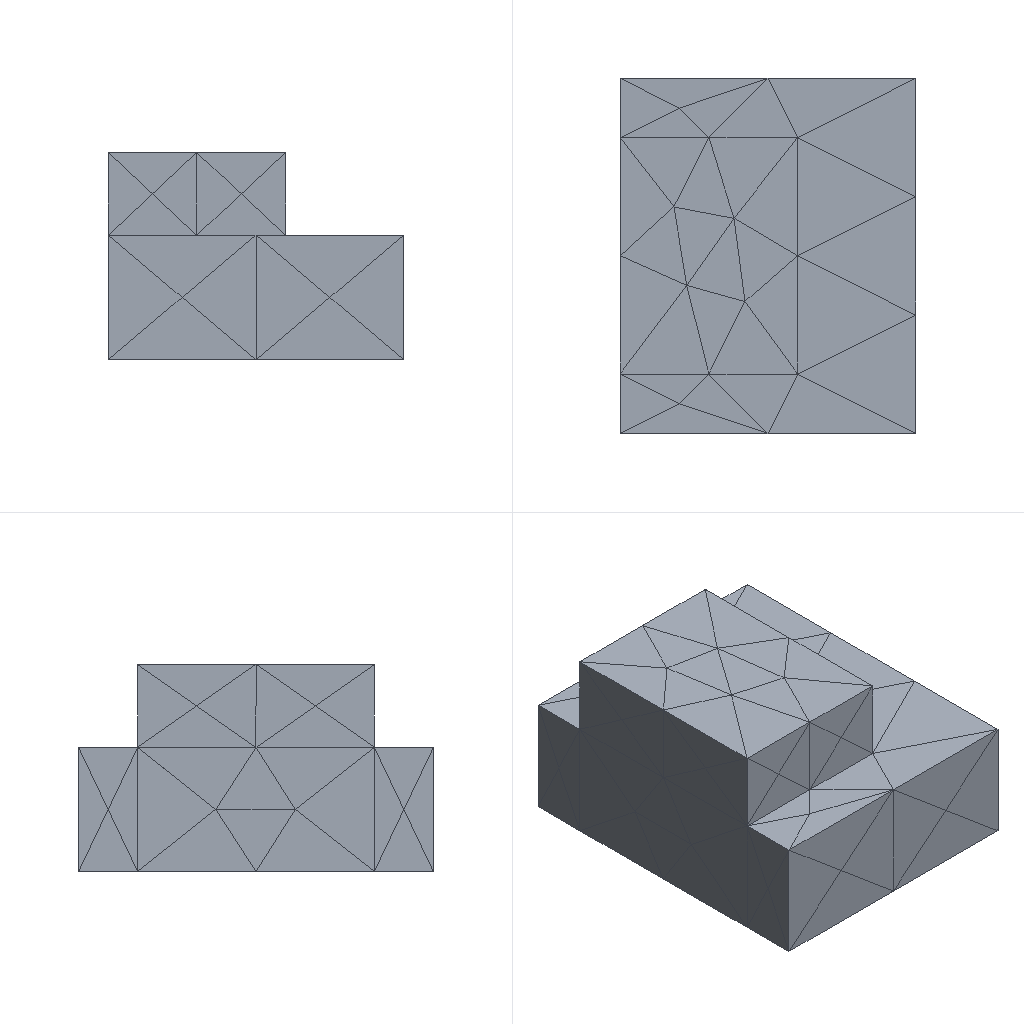Simulation study | ansys mapdl
Set-up summary:
category,name,step,type,value,unit,region
solver,ansys_mapdl
units,mm-N-s-tonne (MPa),,inferred,E=210000 density=
analysis,model,,static
mesh,nodes,,,421
mesh,elements,,,202
element_type,SOLID187,,,202
material,mat 1,,E,210000
material,mat 1,,nu,0.3
load,,model,body load temp,,,all
load,,model,force,"1000 [dir=(0, 0, -1) n=96]",,node list
bc,,model,fixed,"[dofs=UX,UY,UZ n=566]",,node list
Ansys APDL input file, long lists of numbers shortened:
/COM,ANSYS RELEASE 2026 R1           BUILD 26.1      UP20260202       09:11:41
/PREP7
/NOPR
/TITLE,2
ANTYPE, 0
*IF,_CDRDOFF,EQ,1,THEN     !if solid model was read in
_CDRDOFF=             !reset flag, numoffs already performed
*ELSE              !offset database for the following FE model
NUMOFF,NODE,      421
NUMOFF,ELEM,      202
NUMOFF,MAT ,        1
NUMOFF,TYPE,        1
*ENDIF
*SET,_RETURN ,  0.
*SET,_STATUS ,  0.
*SET,_UIQR   ,  96.
*SET,__FLOATPARAMETER__,  421.
DOF,DELETE
ETBLOCK,        1,        1
(2i9,19a9)
        1      187        0        0        0        0        0        0        0        0        0        0        0        0        0        0        0        0        0        0        0
       -1
NBLOCK,6,SOLID,       421,       421
(3i9,6e21.13e3)
        1        0        0 4.3000000000000E+001 8.0000000000000E+000
! (420 more lines like these left out)
N,UNBL,LOC,       -1,
EBLOCK,19,SOLID,       202,       202
(19i10)
         1         1         1         1         0         0         0         0        10         0         1       275         6       276        49       281       282       283       284
! (403 more lines like these left out)
        -1
MPTEMP,UNBL, 1, 1,  0.    ,
MPDATA,UNBL, 1,EX  ,       1, 1,  210000.000    ,
MPTEMP,UNBL, 1, 1,  0.    ,
MPDATA,UNBL, 1,NUXY,       1, 1, 0.3    ,
MPTEMP,UNBL, 1, 1,  0.    ,
MPDATA,UNBL, 1,PRXY,       1, 1, 0.3    ,
EXTOPT,ATTR,      0,      0,      0
EXTOPT,ESIZE,  0,  0.
EXTOPT,ACLEAR,      0
TREF,  0.
IRLF,  0
BFUNIF,TEMP,_TINY
ACEL,  0.    ,  0.    ,  0.
OMEGA,  0.    ,  0.    ,  0.
DOMEGA,  0.    ,  0.    ,  0.
CGLOC,  0.    ,  0.    ,  0.
CGOMEGA,  0.    ,  0.    ,  0.
DCGOMG,  0.    ,  0.    ,  0.
KUSE,     0
TIME,  0.
ALPHAD,  0.
BETAD,  0.
DMPRAT,  0.
DMPSTR,  0.
CRPLIM, 0.1    ,   0
CRPLIM,  0.    ,   1
NCNV,     0, 1.000000000E+12,     0,  0.    ,  0.
NEQIT,     0
ERESX,DEFA
DBLOCK,       566
(i9,a6,2(pg16.9))
        1  UX    0.00000000      0.00000000
! (565 more lines like these left out)
       -1
FBLOCK,        96
(i9,a6,2(pg16.9))
      190  FZ   -10.4166667      0.00000000
! (95 more lines like these left out)
       -1
/GO
FINISH
Results summary:
result,analysis_type_db,,,static,unstated
result,n_sets,,,1,unstated
result,load_steps[0].set,load_step=1,,1,unstated
result,load_steps[0].substep,load_step=1,,1,unstated
result,load_steps[0].time,load_step=1,,1,unstated
result,load_steps[0].freq,load_step=1,,1,unstated
result,load_steps[0].max_usum,load_step=1,,0.000389,unstated
result,load_steps[0].max_seqv,load_step=1,,9.752,unstated
result,load_steps[0].reaction_sum.FX,load_step=1,,-1.47065e-11,unstated
result,load_steps[0].reaction_sum.FY,load_step=1,,-1.01967e-11,unstated
result,load_steps[0].reaction_sum.FZ,load_step=1,,1000,unstated
result,load_steps[0].reaction_sum.MX,load_step=1,,0,unstated
result,load_steps[0].reaction_sum.MY,load_step=1,,0,unstated
result,load_steps[0].reaction_sum.MZ,load_step=1,,0,unstated
result,convergence,,,results present for all listed sets,unstated